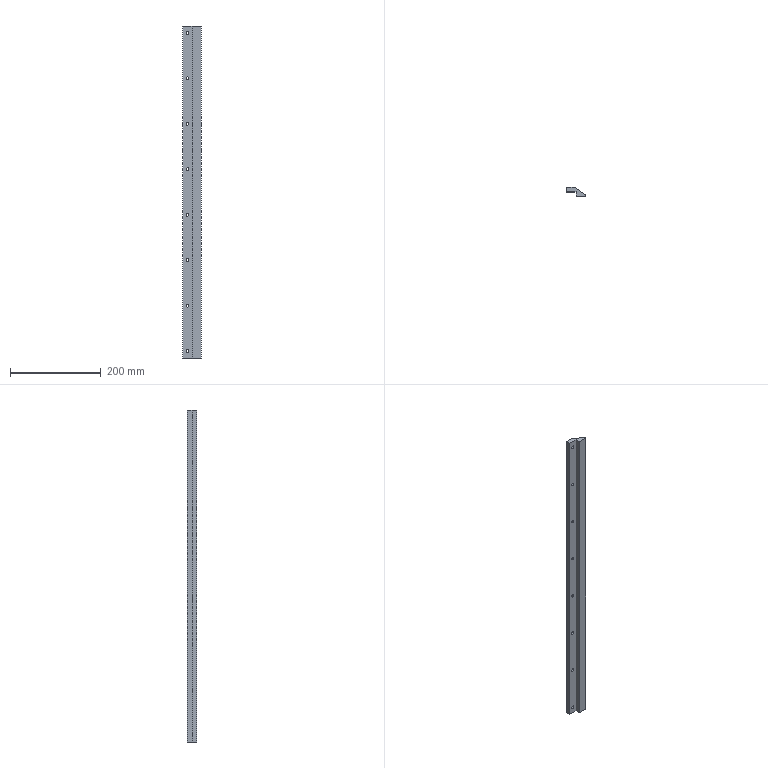NC program | NX | posted with a generic post | part box 40 x 20 x 730 mm
Whole program:
N10 G17 G21 G94 G90
(ZLEVEL_PROFILE , TOOL : D10)
N12 T15 M6
N14 G54
N16 G17 G0 G90 X372.059 Y-0.257 B0. C0. S9500 M3
N18 G43 Z30. H15
N20 Z1.005
N22 G94 G1 Z-0.495 F1000.
N24 X371.301 Y1.055
N26 G3 X370.435 Y1.554 R1.
N28 G1 X365. Y1.553 F2000.
N30 X-365.
N32 X-370.435 Y1.554
N34 X-370.436 Y1.38 Z-0.743
N36 X-370.438 Y1.207 Z-0.991
N38 X-365. Y1.206
N40 X365.
N42 X370.438 Y1.207
N44 X370.439 Y1.033 Z-1.239
N46 X370.44 Y0.86 Z-1.486
N48 X365. Y0.859
N50 X-365.
N52 X-370.441 Y0.86
N54 X-370.442 Y0.686 Z-1.734
N56 X-370.444 Y0.513 Z-1.982
N58 X-365. Y0.512
N60 X365.
N62 X370.443 Y0.513
N64 X370.445 Y0.339 Z-2.23
N66 X370.446 Y0.166 Z-2.477
N68 X365. Y0.165
N70 X-365.
N72 X-370.447 Y0.166
N74 X-370.448 Y-0.008 Z-2.725
N76 X-370.45 Y-0.181 Z-2.973
N78 X-365. Y-0.182
N80 X365.
N82 X370.45 Y-0.181
N84 X370.451 Y-0.355 Z-3.221
N86 X370.453 Y-0.528 Z-3.468
N88 X365. Y-0.529
N90 X-365.
N92 X-370.453 Y-0.528
N94 X-370.454 Y-0.702 Z-3.716
N96 X-370.455 Y-0.875 Z-3.964
N98 X-365. Y-0.876
N100 X365.
N102 X370.456 Y-0.875
N104 X370.457 Y-1.049 Z-4.212
N106 X370.459 Y-1.221 Z-4.459
N108 X365. Y-1.222
N110 X-365.
N112 X-370.458 Y-1.221
N114 X-370.46 Y-1.396 Z-4.707
N116 X-370.461 Y-1.568 Z-4.955
N118 X-365. Y-1.569
N120 X365.
N122 X370.461 Y-1.568
N124 X370.462 Y-1.743 Z-5.203
N126 X370.463 Y-1.915 Z-5.45
N128 X365. Y-1.916
N130 X-365.
N132 X-370.463 Y-1.915
N134 X-370.464 Y-2.09 Z-5.698
N136 X-370.465 Y-2.262 Z-5.946
N138 X-365. Y-2.263
N140 X365.
N142 X370.465 Y-2.262
N144 X370.466 Y-2.437 Z-6.194
N146 X370.467 Y-2.609 Z-6.441
N148 X365. Y-2.61
N150 X-365.
N152 X-370.467 Y-2.609
N154 X-370.468 Y-2.784 Z-6.689
N156 X-370.469 Y-2.956 Z-6.937
N158 X-365. Y-2.957
N160 X365.
N162 X370.469 Y-2.956
N164 X370.47 Y-3.131 Z-7.184
N166 X370.471 Y-3.303 Z-7.432
N168 X365. Y-3.304
N170 X-365.
N172 X-370.471 Y-3.303
N174 X-370.472 Y-3.478 Z-7.68
N176 X-370.473 Y-3.65 Z-7.928
N178 X-365. Y-3.651
N180 X365.
N182 X370.473 Y-3.65
N184 X370.474 Y-3.824 Z-8.175
N186 X370.475 Y-3.997 Z-8.423
N188 X365. Y-3.998
N190 X-365.
N192 X-370.475 Y-3.997
N194 X-370.476 Y-4.171 Z-8.671
N196 Y-4.344 Z-8.919
N198 X-365. Y-4.345
N200 X365.
N202 X370.476 Y-4.344
N204 X370.477 Y-4.518 Z-9.166
N206 X370.478 Y-4.691 Z-9.414
N208 X365. Y-4.692
N210 X-365.
N212 X-370.478 Y-4.691
N214 Y-4.865 Z-9.662
N216 X-370.479 Y-5.038 Z-9.91
N218 X-365. Y-5.039
N220 X365.
N222 X370.479 Y-5.038
N224 Y-5.212 Z-10.157
N226 Y-5.385 Z-10.405
N228 X365. Y-5.386
N230 X-365.
N232 X-370.479 Y-5.385
N234 Y-5.559 Z-10.653
N236 Y-5.732 Z-10.901
N238 X-365. Y-5.733
N240 X365.
N242 X370.479 Y-5.732
N244 Y-5.906 Z-11.148
N246 Y-6.079 Z-11.396
N248 X365. Y-6.08
N250 X-365.
N252 X-370.479 Y-6.079
N254 Y-6.253 Z-11.644
N256 Y-6.426 Z-11.892
N258 X-365. Y-6.427
N260 X365.
N262 X370.479 Y-6.426
N264 Y-6.6 Z-12.139
N266 Y-6.773 Z-12.387
N268 X365.
N270 X-365.
N272 X-370.479
N274 Y-6.947 Z-12.635
N276 Y-7.12 Z-12.882
N278 X-365.
N280 X365.
N282 X370.479
N284 Y-7.294 Z-13.13
N286 Y-7.467 Z-13.378
N288 X365.
N290 X-365.
N292 X-370.479
N294 Y-7.641 Z-13.626
N296 Y-7.814 Z-13.873
N298 X-365.
N300 X365.
N302 X370.479
N304 Y-7.988 Z-14.121
N306 Y-8.161 Z-14.369
N308 X365.
N310 X-365.
N312 X-370.479
N314 Y-8.335 Z-14.617
N316 X-370.478 Y-8.508 Z-14.864
N318 X-365.
N320 X365.
N322 X370.478
N324 X370.477 Y-8.682 Z-15.112
N326 X370.476 Y-8.854 Z-15.36
N328 X365. Y-8.855
N330 X-365.
N332 X-370.477 Y-8.854
N334 X-370.476 Y-9.029 Z-15.608
N336 X-370.475 Y-9.201 Z-15.855
N338 X-365. Y-9.202
N340 X365.
N342 X370.475 Y-9.201
N344 X370.474 Y-9.376 Z-16.103
N346 X370.473 Y-9.548 Z-16.351
N348 X365. Y-9.549
N350 X-365.
N352 X-370.473 Y-9.548
N354 X-370.472 Y-9.722 Z-16.599
N356 X-370.471 Y-9.895 Z-16.846
N358 X-365. Y-9.896
N360 X365.
N362 X370.471 Y-9.895
N364 X370.47 Y-10.069 Z-17.094
N366 X370.469 Y-10.242 Z-17.342
N368 X365. Y-10.243
N370 X-365.
N372 X-370.469 Y-10.242
N374 X-370.468 Y-10.416 Z-17.59
N376 X-370.467 Y-10.589 Z-17.837
N378 X-365. Y-10.59
N380 X365.
N382 X370.467 Y-10.589
N384 X370.466 Y-10.763 Z-18.085
N386 X370.465 Y-10.936 Z-18.333
N388 X365. Y-10.937
N390 X-365.
N392 X-370.465 Y-10.936
N394 X-370.464 Y-11.11 Z-18.58
N396 X-370.463 Y-11.283 Z-18.828
N398 X-365. Y-11.284
N400 X365.
N402 X370.463 Y-11.283
N404 X370.462 Y-11.457 Z-19.076
N406 X370.461 Y-11.63 Z-19.324
N408 X365. Y-11.631
N410 X-365.
N412 X-370.461 Y-11.63
N414 X-370.46 Y-11.804 Z-19.571
N416 X-370.458 Y-11.977 Z-19.819
N418 X-365. Y-11.978
N420 X365.
N422 X370.459 Y-11.977
N424 X370.457 Y-12.151 Z-20.067
N426 X370.456 Y-12.323 Z-20.315
N428 X365. Y-12.324
N430 X-365.
N432 X-370.456 Y-12.323
N434 X-370.454 Y-12.498 Z-20.562
N436 X-370.453 Y-12.67 Z-20.81
N438 X-365. Y-12.671
N440 X365.
N442 X370.453 Y-12.67
N444 X370.451 Y-12.845 Z-21.058
N446 X370.45 Y-13.017 Z-21.306
N448 X365. Y-13.018
N450 X-365.
N452 X-370.45 Y-13.017
N454 X-370.448 Y-13.192 Z-21.553
N456 X-370.447 Y-13.364 Z-21.801
N458 X-365. Y-13.365
N460 X365.
N462 X370.447 Y-13.364
N464 X370.445 Y-13.539 Z-22.049
N466 X370.444 Y-13.711 Z-22.297
N468 X365. Y-13.712
N470 X-365.
N472 X-370.444 Y-13.711
N474 X-370.442 Y-13.886 Z-22.544
N476 X-370.441 Y-14.058 Z-22.792
N478 X-365. Y-14.059
N480 X365.
N482 X370.441 Y-14.058
N484 X370.439 Y-14.233 Z-23.04
N486 X370.438 Y-14.405 Z-23.288
N488 X365. Y-14.406
N490 X-365.
N492 X-370.438 Y-14.405
N494 X-370.436 Y-14.58 Z-23.535
N496 X-370.435 Y-14.752 Z-23.783
N498 X-365. Y-14.753
N500 X365.
N502 X370.435 Y-14.752
N504 X370.433 Y-14.927 Z-24.031
N506 X370.432 Y-15.099 Z-24.279
N508 X-370.431
N510 G3 X-371.297 Y-15.599 R1.
N512 G1 X-372.055 Y-16.911
N514 Z-22.779
N516 G0 Z30.
N518 M5
(ZLEVEL_PROFILE_COPY , TOOL : D6R0.5)
N520 T16 M6
N522 G54
N524 G17 G0 G90 X365.969 Y2.951 B0. C0. S9500 M3
N526 G43 Z30. H16
N528 Z1.2
N530 G94 G1 Z-0.3 F1000.
N532 X365.52 Y3.73
N534 G3 X365. Y4.03 R0.6
N536 G1 X-365. F2500.
N538 Y3.96 Z-0.4
N540 X365.
N542 Y3.89 Z-0.5
N544 X-365.
N546 Y3.82 Z-0.6
N548 X365.
N550 Y3.75 Z-0.7
N552 X-365.
N554 Y3.68 Z-0.8
N556 X365.
N558 Y3.61 Z-0.9
N560 X-365.
N562 Y3.54 Z-1.
N564 X365.
N566 Y3.469 Z-1.1
N568 X-365.
N570 Y3.399 Z-1.2
N572 X365.
N574 Y3.329 Z-1.3
N576 X-365.
N578 Y3.259 Z-1.4
N580 X365.
N582 Y3.189 Z-1.5
N584 X-365.
N586 Y3.119 Z-1.6
N588 X365.
N590 Y3.049 Z-1.7
N592 X-365.
N594 Y2.979 Z-1.8
N596 X365.
N598 Y2.909 Z-1.9
N600 X-365.
N602 Y2.839 Z-2.
N604 X365.
N606 Y2.769 Z-2.1
N608 X-365.
N610 Y2.699 Z-2.2
N612 X365.
N614 Y2.629 Z-2.3
N616 X-365.
N618 Y2.559 Z-2.4
N620 X365.
N622 Y2.489 Z-2.5
N624 X-365.
N626 Y2.419 Z-2.6
N628 X365.
N630 Y2.349 Z-2.7
N632 X-365.
N634 Y2.279 Z-2.8
N636 X365.
N638 Y2.209 Z-2.9
N640 X-365.
N642 Y2.139 Z-3.
N644 X365.
N646 Y2.069 Z-3.1
N648 X-365.
N650 Y1.999 Z-3.2
N652 X365.
N654 Y1.929 Z-3.3
N656 X-365.
N658 Y1.859 Z-3.4
N660 X365.
N662 Y1.789 Z-3.5
N664 X-365.
N666 Y1.719 Z-3.6
N668 X365.
N670 Y1.649 Z-3.7
N672 X-365.
N674 Y1.579 Z-3.8
N676 X365.
N678 Y1.509 Z-3.9
N680 X-365.
N682 Y1.439 Z-4.
N684 X365.
N686 Y1.369 Z-4.1
N688 X-365.
N690 Y1.299 Z-4.2
N692 X365.
N694 Y1.229 Z-4.3
N696 X-365.
N698 Y1.159 Z-4.4
N700 X365.
N702 Y1.089 Z-4.5
N704 X-365.
N706 Y1.019 Z-4.6
N708 X365.
N710 Y0.949 Z-4.7
N712 X-365.
N714 Y0.879 Z-4.8
N716 X365.
N718 Y0.809 Z-4.9
N720 X-365.
N722 Y0.739 Z-5.
N724 X365.
N726 Y0.669 Z-5.1
N728 X-365.
N730 Y0.599 Z-5.2
N732 X365.
N734 Y0.529 Z-5.3
N736 X-365.
N738 Y0.459 Z-5.4
N740 X365.
N742 Y0.389 Z-5.5
N744 X-365.
N746 Y0.319 Z-5.6
N748 X365.
N750 Y0.249 Z-5.7
N752 X-365.
N754 Y0.179 Z-5.8
N756 X365.
N758 Y0.108 Z-5.9
N760 X-365.
N762 Y0.038 Z-6.
N764 X365.
N766 Y-0.032 Z-6.1
N768 X-365.
N770 Y-0.102 Z-6.2
N772 X365.
N774 Y-0.172 Z-6.3
N776 X-365.
N778 Y-0.242 Z-6.4
N780 X365.
N782 Y-0.312 Z-6.5
N784 X-365.
N786 Y-0.382 Z-6.6
N788 X365.
N790 Y-0.452 Z-6.7
N792 X-365.
N794 Y-0.522 Z-6.8
N796 X365.
N798 Y-0.592 Z-6.9
N800 X-365.
N802 Y-0.662 Z-7.
N804 X365.
N806 Y-0.732 Z-7.1
N808 X-365.
N810 Y-0.802 Z-7.2
N812 X365.
N814 Y-0.872 Z-7.3
N816 X-365.
N818 Y-0.942 Z-7.4
N820 X365.
N822 Y-1.012 Z-7.5
N824 X-365.
N826 Y-1.082 Z-7.6
N828 X365.
N830 Y-1.152 Z-7.7
N832 X-365.
N834 Y-1.222 Z-7.8
N836 X365.
N838 Y-1.292 Z-7.9
N840 X-365.
N842 Y-1.362 Z-8.
N844 X365.
N846 Y-1.432 Z-8.1
N848 X-365.
N850 Y-1.502 Z-8.2
N852 X365.
N854 Y-1.572 Z-8.3
N856 X-365.
N858 Y-1.642 Z-8.4
N860 X365.
N862 Y-1.712 Z-8.5
N864 X-365.
N866 Y-1.782 Z-8.6
N868 X365.
N870 Y-1.852 Z-8.7
N872 X-365.
N874 Y-1.922 Z-8.8
N876 X365.
N878 Y-1.992 Z-8.9
N880 X-365.
N882 Y-2.062 Z-9.
N884 X365.
N886 Y-2.132 Z-9.1
N888 X-365.
N890 Y-2.202 Z-9.2
N892 X365.
N894 Y-2.272 Z-9.3
N896 X-365.
N898 Y-2.342 Z-9.4
N900 X365.
N902 Y-2.412 Z-9.5
N904 X-365.
N906 Y-2.482 Z-9.6
N908 X365.
N910 Y-2.552 Z-9.7
N912 X-365.
N914 Y-2.622 Z-9.8
N916 X365.
N918 Y-2.692 Z-9.9
N920 X-365.
N922 Y-2.762 Z-10.
N924 X365.
N926 Y-2.832 Z-10.1
N928 X-365.
N930 Y-2.902 Z-10.2
N932 X365.
N934 Y-2.972 Z-10.3
N936 X-365.
N938 Y-3.042 Z-10.4
N940 X365.
N942 Y-3.112 Z-10.5
N944 X-365.
N946 Y-3.182 Z-10.6
N948 X365.
N950 Y-3.253 Z-10.7
N952 X-365.
N954 Y-3.323 Z-10.8
N956 X365.
N958 Y-3.393 Z-10.9
N960 X-365.
N962 Y-3.463 Z-11.
N964 X365.
N966 Y-3.533 Z-11.1
N968 X-365.
N970 Y-3.603 Z-11.2
N972 X365.
N974 Y-3.673 Z-11.3
N976 X-365.
N978 Y-3.743 Z-11.4
N980 X365.
N982 Y-3.813 Z-11.5
N984 X-365.
N986 Y-3.883 Z-11.6
N988 X365.
N990 Y-3.953 Z-11.7
N992 X-365.
N994 Y-4.023 Z-11.8
N996 X365.
N998 Y-4.093 Z-11.9
N1000 X-365.
N1002 Y-4.163 Z-12.
N1004 X365.
N1006 Y-4.233 Z-12.1
N1008 X-365.
N1010 Y-4.303 Z-12.2
N1012 X365.
N1014 Y-4.373 Z-12.3
N1016 X-365.
N1018 Y-4.443 Z-12.4
N1020 X365.
N1022 Y-4.513 Z-12.5
N1024 X-365.
N1026 Y-4.583 Z-12.6
N1028 X365.
N1030 Y-4.653 Z-12.7
N1032 X-365.
N1034 Y-4.723 Z-12.8
N1036 X365.
N1038 Y-4.793 Z-12.9
N1040 X-365.
N1042 Y-4.863 Z-13.
N1044 X365.
N1046 Y-4.933 Z-13.1
N1048 X-365.
N1050 Y-5.003 Z-13.2
N1052 X365.
N1054 Y-5.073 Z-13.3
N1056 X-365.
N1058 Y-5.143 Z-13.4
N1060 X365.
N1062 Y-5.213 Z-13.5
N1064 X-365.
N1066 Y-5.283 Z-13.6
N1068 X365.
N1070 Y-5.353 Z-13.7
N1072 X-365.
N1074 Y-5.423 Z-13.8
N1076 X365.
N1078 Y-5.493 Z-13.9
N1080 X-365.
N1082 Y-5.563 Z-14.
N1084 X365.
N1086 Y-5.633 Z-14.1
N1088 X-365.
N1090 Y-5.703 Z-14.2
N1092 X365.
N1094 Y-5.773 Z-14.3
N1096 X-365.
N1098 Y-5.843 Z-14.4
N1100 X365.
N1102 Y-5.913 Z-14.5
N1104 X-365.
N1106 Y-5.983 Z-14.6
N1108 X365.
N1110 Y-6.053 Z-14.7
N1112 X-365.
N1114 Y-6.123 Z-14.8
N1116 X365.
N1118 Y-6.193 Z-14.9
N1120 X-365.
N1122 Y-6.263 Z-15.
N1124 X365.
N1126 Y-6.333 Z-15.1
N1128 X-365.
N1130 Y-6.403 Z-15.2
N1132 X365.
N1134 Y-6.473 Z-15.3
N1136 X-365.
N1138 Y-6.543 Z-15.4
N1140 X365.
N1142 Y-6.614 Z-15.5
N1144 X-365.
N1146 Y-6.684 Z-15.6
N1148 X365.
N1150 Y-6.754 Z-15.7
N1152 X-365.
N1154 Y-6.824 Z-15.8
N1156 X365.
N1158 Y-6.894 Z-15.9
N1160 X-365.
N1162 Y-6.964 Z-16.
N1164 X365.
N1166 Y-7.034 Z-16.1
N1168 X-365.
N1170 Y-7.104 Z-16.2
N1172 X365.
N1174 Y-7.174 Z-16.3
N1176 X-365.
N1178 Y-7.244 Z-16.4
N1180 X365.
N1182 Y-7.314 Z-16.5
N1184 X-365.
N1186 Y-7.384 Z-16.6
N1188 X365.
N1190 Y-7.454 Z-16.7
N1192 X-365.
N1194 Y-7.524 Z-16.8
N1196 X365.
N1198 Y-7.594 Z-16.9
N1200 X-365.
N1202 Y-7.664 Z-17.
N1204 X365.
N1206 Y-7.734 Z-17.1
N1208 X-365.
N1210 Y-7.804 Z-17.2
N1212 X365.
N1214 Y-7.874 Z-17.3
N1216 X-365.
N1218 Y-7.944 Z-17.4
N1220 X365.
N1222 Y-8.014 Z-17.5
N1224 X-365.
N1226 Y-8.084 Z-17.6
N1228 X365.
N1230 Y-8.154 Z-17.7
N1232 X-365.
N1234 Y-8.224 Z-17.8
N1236 X365.
N1238 Y-8.294 Z-17.9
N1240 X-365.
N1242 Y-8.364 Z-18.
N1244 X365.
N1246 Y-8.434 Z-18.1
N1248 X-365.
N1250 Y-8.504 Z-18.2
N1252 X365.
N1254 Y-8.574 Z-18.3
N1256 X-365.
N1258 Y-8.644 Z-18.4
N1260 X365.
N1262 Y-8.714 Z-18.5
N1264 X-365.
N1266 Y-8.784 Z-18.6
N1268 X365.
N1270 Y-8.854 Z-18.7
N1272 X-365.
N1274 Y-8.924 Z-18.8
N1276 X365.
N1278 Y-8.994 Z-18.9
N1280 X-365.
N1282 Y-9.064 Z-19.
N1284 X365.
N1286 Y-9.134 Z-19.1
N1288 X-365.
N1290 Y-9.204 Z-19.2
N1292 X365.
N1294 Y-9.274 Z-19.3
N1296 X-365.
N1298 Y-9.344 Z-19.4
N1300 X365.
N1302 Y-9.414 Z-19.5
N1304 X-365.
N1306 Y-9.484 Z-19.6
N1308 X365.
N1310 Y-9.554 Z-19.7
N1312 X-365.
N1314 Y-9.624 Z-19.8
N1316 X365.
N1318 Y-9.694 Z-19.9
N1320 X-365.
N1322 Y-9.729 Z-19.95
N1324 Y-9.763 Z-20.
N1326 X365.
N1328 Y-9.799 Z-20.05
N1330 Y-9.834 Z-20.1
N1332 X-365.
N1334 Y-9.904 Z-20.2
N1336 X365.
N1338 Y-9.974 Z-20.3
N1340 X-365.
N1342 Y-10.045 Z-20.4
N1344 X365.
N1346 Y-10.115 Z-20.5
N1348 X-365.
N1350 Y-10.185 Z-20.6
N1352 X365.
N1354 Y-10.255 Z-20.7
N1356 X-365.
N1358 Y-10.325 Z-20.8
N1360 X365.
N1362 Y-10.395 Z-20.9
N1364 X-365.
N1366 Y-10.465 Z-21.
N1368 X365.
N1370 Y-10.535 Z-21.1
N1372 X-365.
N1374 Y-10.605 Z-21.2
N1376 X365.
N1378 Y-10.675 Z-21.3
N1380 X-365.
N1382 Y-10.745 Z-21.4
N1384 X365.
N1386 Y-10.815 Z-21.5
N1388 X-365.
N1390 Y-10.885 Z-21.6
N1392 X365.
N1394 Y-10.955 Z-21.7
N1396 X-365.
N1398 Y-11.025 Z-21.8
N1400 X365.
N1402 Y-11.095 Z-21.9
N1404 X-365.
N1406 Y-11.165 Z-22.
N1408 X365.
N1410 Y-11.235 Z-22.1
N1412 X-365.
N1414 Y-11.305 Z-22.2
N1416 X365.
N1418 Y-11.375 Z-22.3
N1420 X-365.
N1422 Y-11.445 Z-22.4
N1424 X365.
N1426 Y-11.515 Z-22.5
N1428 X-365.
N1430 Y-11.585 Z-22.6
N1432 X365.
N1434 Y-11.655 Z-22.7
N1436 X-365.
N1438 Y-11.725 Z-22.8
N1440 X365.
N1442 Y-11.795 Z-22.9
N1444 X-365.
N1446 Y-11.865 Z-23.
N1448 X365.
N1450 Y-11.935 Z-23.1
N1452 X-365.
N1454 Y-12.005 Z-23.2
N1456 X365.
N1458 Y-12.075 Z-23.3
N1460 X-365.
N1462 Y-12.145 Z-23.4
N1464 X365.
N1466 Y-12.215 Z-23.5
N1468 X-365.
N1470 Y-12.285 Z-23.6
N1472 X365.
N1474 Y-12.355 Z-23.7
N1476 X-365.
N1478 Y-12.425 Z-23.8
N1480 X365.
N1482 Y-12.495 Z-23.9
N1484 X-365.
N1486 Y-12.565 Z-24.
N1488 X365.
N1490 Y-12.635 Z-24.1
N1492 X-365.
N1494 Y-12.705 Z-24.2
N1496 X365.
N1498 Y-12.775 Z-24.3
N1500 X-365.
N1502 Y-12.845 Z-24.4
N1504 X365.
N1506 G2 X365.52 Y-13.145 R0.6
N1508 G1 X365.971 Y-13.927
N1510 Z-22.9
N1512 G0 Z30.
N1514 M5
N1516 M2